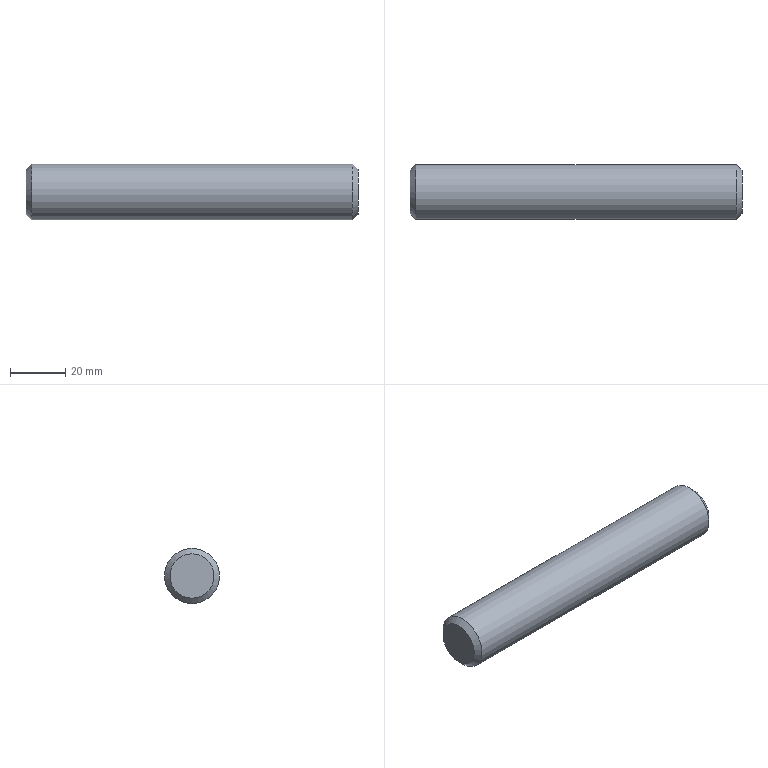Part | STEP file | solid 219 | 1 solid | 5 faces | box 120 x 20 x 20 mm | volume 37465 mm3 | plane 2 | cone 2 | cylinder 1 | commonest cylinder face diameters 20 x1